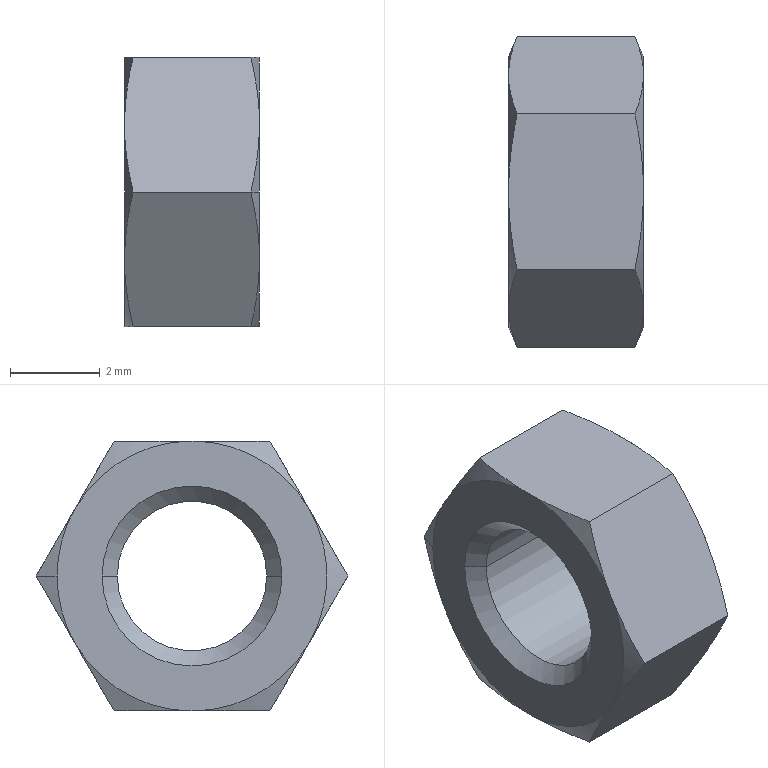Part | SolidWorks | features RefAxis 3, 3DProfileFeature 1, ICE 1, Revolution 1, Scale 1 | 1 solid | 28 faces | box 3 x 6.928 x 6 mm | volume 65.89 mm3 | cone 18 | plane 8 | cylinder 2 | commonest cylinder face diameters 3.324 x2
STEP:
#1=CARTESIAN_POINT('',(1.162,1.662,0.));
#2=VERTEX_POINT('',#1);
#3=CARTESIAN_POINT('',(1.162,-1.662,0.));
#4=VERTEX_POINT('',#3);
#5=CARTESIAN_POINT('',(1.162,0.,0.));
#6=DIRECTION('',(-1.,0.,0.));
#7=DIRECTION('',(0.,-1.,0.));
#8=AXIS2_PLACEMENT_3D('',#5,#6,#7);
#9=CIRCLE('',#8,1.662);
#10=EDGE_CURVE('',#2,#4,#9,.T.);
#11=ORIENTED_EDGE('',*,*,#10,.T.);
#12=CARTESIAN_POINT('',(1.5,-2.,0.));
#13=VERTEX_POINT('',#12);
#14=CARTESIAN_POINT('',(1.162,-1.662,0.));
#15=DIRECTION('',(0.7071,-0.7071,0.));
#16=VECTOR('',#15,1000.);
#17=LINE('',#14,#16);
#18=EDGE_CURVE('',#4,#13,#17,.T.);
#19=ORIENTED_EDGE('',*,*,#18,.T.);
#20=CARTESIAN_POINT('',(1.5,2.,0.));
#21=VERTEX_POINT('',#20);
#22=CARTESIAN_POINT('',(1.5,0.,0.));
#23=DIRECTION('',(-1.,0.,0.));
#24=DIRECTION('',(0.,-1.,0.));
#25=AXIS2_PLACEMENT_3D('',#22,#23,#24);
#26=CIRCLE('',#25,2.);
#27=EDGE_CURVE('',#21,#13,#26,.T.);
#28=ORIENTED_EDGE('',*,*,#27,.F.);
#29=CARTESIAN_POINT('',(1.162,1.662,0.));
#30=DIRECTION('',(0.7071,0.7071,0.));
#31=VECTOR('',#30,1000.);
#32=LINE('',#29,#31);
#33=EDGE_CURVE('',#2,#21,#32,.T.);
#34=ORIENTED_EDGE('',*,*,#33,.F.);
#35=EDGE_LOOP('',(#11,#19,#28,#34));
#36=FACE_OUTER_BOUND('',#35,.T.);
#37=CARTESIAN_POINT('',(1.162,0.,0.));
#38=DIRECTION('',(1.,0.,0.));
#39=DIRECTION('',(0.,1.,0.));
#40=AXIS2_PLACEMENT_3D('',#37,#38,#39);
#41=CONICAL_SURFACE('',#40,1.662,0.7854);
#42=ADVANCED_FACE('',(#36),#41,.F.);
#43=ORIENTED_EDGE('',*,*,#10,.F.);
#44=CARTESIAN_POINT('',(-1.162,1.662,0.));
#45=VERTEX_POINT('',#44);
#46=CARTESIAN_POINT('',(1.5,1.662,0.));
#47=DIRECTION('',(-1.,0.,0.));
#48=VECTOR('',#47,1000.);
#49=LINE('',#46,#48);
#50=EDGE_CURVE('',#2,#45,#49,.T.);
#51=ORIENTED_EDGE('',*,*,#50,.T.);
#52=CARTESIAN_POINT('',(-1.162,-1.662,0.));
#53=VERTEX_POINT('',#52);
#54=CARTESIAN_POINT('',(-1.162,0.,0.));
#55=DIRECTION('',(-1.,0.,0.));
#56=DIRECTION('',(0.,-1.,0.));
#57=AXIS2_PLACEMENT_3D('',#54,#55,#56);
#58=CIRCLE('',#57,1.662);
#59=EDGE_CURVE('',#45,#53,#58,.T.);
#60=ORIENTED_EDGE('',*,*,#59,.T.);
#61=CARTESIAN_POINT('',(1.5,-1.662,0.));
#62=DIRECTION('',(-1.,0.,0.));
#63=VECTOR('',#62,1000.);
#64=LINE('',#61,#63);
#65=EDGE_CURVE('',#4,#53,#64,.T.);
#66=ORIENTED_EDGE('',*,*,#65,.F.);
#67=EDGE_LOOP('',(#43,#51,#60,#66));
#68=FACE_OUTER_BOUND('',#67,.T.);
#69=CARTESIAN_POINT('',(1.5,0.,0.));
#70=DIRECTION('',(-1.,0.,0.));
#71=DIRECTION('',(0.,-1.,0.));
#72=AXIS2_PLACEMENT_3D('',#69,#70,#71);
#73=CYLINDRICAL_SURFACE('',#72,1.662);
#74=ADVANCED_FACE('',(#68),#73,.F.);
#75=ORIENTED_EDGE('',*,*,#59,.F.);
#76=CARTESIAN_POINT('',(-1.5,2.,0.));
#77=VERTEX_POINT('',#76);
#78=CARTESIAN_POINT('',(-1.5,2.,0.));
#79=DIRECTION('',(-0.7071,0.7071,0.));
#80=VECTOR('',#79,1000.);
#81=LINE('',#78,#80);
#82=EDGE_CURVE('',#45,#77,#81,.T.);
#83=ORIENTED_EDGE('',*,*,#82,.T.);
#84=CARTESIAN_POINT('',(-1.5,-2.,0.));
#85=VERTEX_POINT('',#84);
#86=CARTESIAN_POINT('',(-1.5,0.,0.));
#87=DIRECTION('',(-1.,0.,0.));
#88=DIRECTION('',(0.,-1.,0.));
#89=AXIS2_PLACEMENT_3D('',#86,#87,#88);
#90=CIRCLE('',#89,2.);
#91=EDGE_CURVE('',#77,#85,#90,.T.);
#92=ORIENTED_EDGE('',*,*,#91,.T.);
#93=CARTESIAN_POINT('',(-1.5,-2.,0.));
#94=DIRECTION('',(-0.7071,-0.7071,0.));
#95=VECTOR('',#94,1000.);
#96=LINE('',#93,#95);
#97=EDGE_CURVE('',#53,#85,#96,.T.);
#98=ORIENTED_EDGE('',*,*,#97,.F.);
#99=EDGE_LOOP('',(#75,#83,#92,#98));
#100=FACE_OUTER_BOUND('',#99,.T.);
#101=CARTESIAN_POINT('',(-1.5,0.,0.));
#102=DIRECTION('',(-1.,0.,0.));
#103=DIRECTION('',(0.,-1.,0.));
#104=AXIS2_PLACEMENT_3D('',#101,#102,#103);
#105=CONICAL_SURFACE('',#104,2.,0.7854);
#106=ADVANCED_FACE('',(#100),#105,.F.);
#107=CARTESIAN_POINT('',(1.5,-2.598,-1.5));
#108=VERTEX_POINT('',#107);
#109=CARTESIAN_POINT('',(1.5,-3.,0.));
#110=VERTEX_POINT('',#109);
#111=CARTESIAN_POINT('',(1.5,0.,0.));
#112=DIRECTION('',(-1.,0.,0.));
#113=DIRECTION('',(0.,-1.,0.));
#114=AXIS2_PLACEMENT_3D('',#111,#112,#113);
#115=CIRCLE('',#114,3.);
#116=EDGE_CURVE('',#108,#110,#115,.T.);
#117=ORIENTED_EDGE('',*,*,#116,.T.);
#118=CARTESIAN_POINT('',(1.308,-3.464,0.));
#119=VERTEX_POINT('',#118);
#120=CARTESIAN_POINT('',(1.5,-3.,0.));
#121=DIRECTION('',(-0.3827,-0.9239,0.));
#122=VECTOR('',#121,1000.);
#123=LINE('',#120,#122);
#124=EDGE_CURVE('',#110,#119,#123,.T.);
#125=ORIENTED_EDGE('',*,*,#124,.T.);
#126=CARTESIAN_POINT('',(1.5,-2.598,-1.5));
#127=CARTESIAN_POINT('',(1.5,-2.742,-1.25));
#128=CARTESIAN_POINT('',(1.482,-2.887,-1.));
#129=CARTESIAN_POINT('',(1.416,-3.176,-0.499));
#130=CARTESIAN_POINT('',(1.367,-3.321,-0.2483));
#131=CARTESIAN_POINT('',(1.308,-3.464,0.));
#132=B_SPLINE_CURVE_WITH_KNOTS('',3,(#126,#127,#128,#129,#130,#131),.UNSPECIFIED.,.F.,.F.,(4,2,4),(0.001738,0.002602,0.003466),.UNSPECIFIED.);
#133=EDGE_CURVE('',#108,#119,#132,.T.);
#134=ORIENTED_EDGE('',*,*,#133,.F.);
#135=EDGE_LOOP('',(#117,#125,#134));
#136=FACE_OUTER_BOUND('',#135,.T.);
#137=CARTESIAN_POINT('',(1.5,0.,0.));
#138=DIRECTION('',(-1.,0.,0.));
#139=DIRECTION('',(0.,-1.,0.));
#140=AXIS2_PLACEMENT_3D('',#137,#138,#139);
#141=CONICAL_SURFACE('',#140,3.,1.178);
#142=ADVANCED_FACE('',(#136),#141,.T.);
#143=CARTESIAN_POINT('',(-1.5,3.,0.));
#144=VERTEX_POINT('',#143);
#145=CARTESIAN_POINT('',(-1.5,2.598,-1.5));
#146=VERTEX_POINT('',#145);
#147=CARTESIAN_POINT('',(-1.5,0.,0.));
#148=DIRECTION('',(-1.,0.,0.));
#149=DIRECTION('',(0.,-1.,0.));
#150=AXIS2_PLACEMENT_3D('',#147,#148,#149);
#151=CIRCLE('',#150,3.);
#152=EDGE_CURVE('',#144,#146,#151,.T.);
#153=ORIENTED_EDGE('',*,*,#152,.F.);
#154=CARTESIAN_POINT('',(-1.308,3.464,0.));
#155=VERTEX_POINT('',#154);
#156=CARTESIAN_POINT('',(0.,6.621,0.));
#157=DIRECTION('',(0.3827,0.9239,0.));
#158=VECTOR('',#157,1000.);
#159=LINE('',#156,#158);
#160=EDGE_CURVE('',#144,#155,#159,.T.);
#161=ORIENTED_EDGE('',*,*,#160,.T.);
#162=CARTESIAN_POINT('',(-1.5,2.598,-1.5));
#163=CARTESIAN_POINT('',(-1.5,2.742,-1.25));
#164=CARTESIAN_POINT('',(-1.482,2.887,-1.));
#165=CARTESIAN_POINT('',(-1.416,3.176,-0.499));
#166=CARTESIAN_POINT('',(-1.367,3.321,-0.2483));
#167=CARTESIAN_POINT('',(-1.308,3.464,0.));
#168=B_SPLINE_CURVE_WITH_KNOTS('',3,(#162,#163,#164,#165,#166,#167),.UNSPECIFIED.,.F.,.F.,(4,2,4),(0.001738,0.002602,0.003466),.UNSPECIFIED.);
#169=EDGE_CURVE('',#146,#155,#168,.T.);
#170=ORIENTED_EDGE('',*,*,#169,.F.);
#171=EDGE_LOOP('',(#153,#161,#170));
#172=FACE_OUTER_BOUND('',#171,.T.);
#173=CARTESIAN_POINT('',(0.,0.,0.));
#174=DIRECTION('',(1.,0.,0.));
#175=DIRECTION('',(0.,1.,0.));
#176=AXIS2_PLACEMENT_3D('',#173,#174,#175);
#177=CONICAL_SURFACE('',#176,6.621,1.178);
#178=ADVANCED_FACE('',(#172),#177,.T.);
#179=CARTESIAN_POINT('',(-1.308,1.732,-3.));
#180=VERTEX_POINT('',#179);
#181=CARTESIAN_POINT('',(-1.308,1.732,-3.));
#182=CARTESIAN_POINT('',(-1.427,2.02,-2.502));
#183=CARTESIAN_POINT('',(-1.5,2.308,-2.002));
#184=CARTESIAN_POINT('',(-1.5,2.598,-1.5));
#185=B_SPLINE_CURVE_WITH_KNOTS('',3,(#181,#182,#183,#184),.UNSPECIFIED.,.F.,.F.,(4,4),(0.000000116,0.001738),.UNSPECIFIED.);
#186=EDGE_CURVE('',#180,#146,#185,.T.);
#187=ORIENTED_EDGE('',*,*,#186,.F.);
#188=CARTESIAN_POINT('',(-1.5,0.,-3.));
#189=VERTEX_POINT('',#188);
#190=CARTESIAN_POINT('',(-1.5,0.,-3.));
#191=CARTESIAN_POINT('',(-1.5,0.2891,-3.));
#192=CARTESIAN_POINT('',(-1.482,0.5782,-3.));
#193=CARTESIAN_POINT('',(-1.416,1.157,-3.));
#194=CARTESIAN_POINT('',(-1.367,1.447,-3.));
#195=CARTESIAN_POINT('',(-1.308,1.732,-3.));
#196=B_SPLINE_CURVE_WITH_KNOTS('',3,(#190,#191,#192,#193,#194,#195),.UNSPECIFIED.,.F.,.F.,(4,2,4),(0.004788,0.005662,0.006536),.UNSPECIFIED.);
#197=EDGE_CURVE('',#189,#180,#196,.T.);
#198=ORIENTED_EDGE('',*,*,#197,.F.);
#199=CARTESIAN_POINT('',(-1.5,0.,0.));
#200=DIRECTION('',(-1.,0.,0.));
#201=DIRECTION('',(0.,-1.,0.));
#202=AXIS2_PLACEMENT_3D('',#199,#200,#201);
#203=CIRCLE('',#202,3.);
#204=EDGE_CURVE('',#146,#189,#203,.T.);
#205=ORIENTED_EDGE('',*,*,#204,.F.);
#206=EDGE_LOOP('',(#187,#198,#205));
#207=FACE_OUTER_BOUND('',#206,.T.);
#208=CARTESIAN_POINT('',(0.,0.,0.));
#209=DIRECTION('',(1.,0.,0.));
#210=DIRECTION('',(0.,1.,0.));
#211=AXIS2_PLACEMENT_3D('',#208,#209,#210);
#212=CONICAL_SURFACE('',#211,6.621,1.178);
#213=ADVANCED_FACE('',(#207),#212,.T.);
#214=ORIENTED_EDGE('',*,*,#160,.F.);
#215=CARTESIAN_POINT('',(-1.5,2.598,1.5));
#216=VERTEX_POINT('',#215);
#217=CARTESIAN_POINT('',(-1.5,0.,0.));
#218=DIRECTION('',(-1.,0.,0.));
#219=DIRECTION('',(0.,-1.,0.));
#220=AXIS2_PLACEMENT_3D('',#217,#218,#219);
#221=CIRCLE('',#220,3.);
#222=EDGE_CURVE('',#216,#144,#221,.T.);
#223=ORIENTED_EDGE('',*,*,#222,.F.);
#224=CARTESIAN_POINT('',(-1.308,3.464,0.));
#225=CARTESIAN_POINT('',(-1.427,3.176,0.4982));
#226=CARTESIAN_POINT('',(-1.5,2.888,0.9979));
#227=CARTESIAN_POINT('',(-1.5,2.598,1.5));
#228=B_SPLINE_CURVE_WITH_KNOTS('',3,(#224,#225,#226,#227),.UNSPECIFIED.,.F.,.F.,(4,4),(0.000000116,0.001738),.UNSPECIFIED.);
#229=EDGE_CURVE('',#155,#216,#228,.T.);
#230=ORIENTED_EDGE('',*,*,#229,.F.);
#231=EDGE_LOOP('',(#214,#223,#230));
#232=FACE_OUTER_BOUND('',#231,.T.);
#233=CARTESIAN_POINT('',(0.,0.,0.));
#234=DIRECTION('',(1.,0.,0.));
#235=DIRECTION('',(0.,1.,0.));
#236=AXIS2_PLACEMENT_3D('',#233,#234,#235);
#237=CONICAL_SURFACE('',#236,6.621,1.178);
#238=ADVANCED_FACE('',(#232),#237,.T.);
#239=CARTESIAN_POINT('',(-1.308,1.732,3.));
#240=VERTEX_POINT('',#239);
#241=CARTESIAN_POINT('',(-1.5,2.598,1.5));
#242=CARTESIAN_POINT('',(-1.5,2.454,1.75));
#243=CARTESIAN_POINT('',(-1.482,2.31,2.));
#244=CARTESIAN_POINT('',(-1.416,2.02,2.501));
#245=CARTESIAN_POINT('',(-1.367,1.875,2.752));
#246=CARTESIAN_POINT('',(-1.308,1.732,3.));
#247=B_SPLINE_CURVE_WITH_KNOTS('',3,(#241,#242,#243,#244,#245,#246),.UNSPECIFIED.,.F.,.F.,(4,2,4),(0.001738,0.002602,0.003466),.UNSPECIFIED.);
#248=EDGE_CURVE('',#216,#240,#247,.T.);
#249=ORIENTED_EDGE('',*,*,#248,.F.);
#250=CARTESIAN_POINT('',(-1.5,0.,3.));
#251=VERTEX_POINT('',#250);
#252=CARTESIAN_POINT('',(-1.5,0.,0.));
#253=DIRECTION('',(-1.,0.,0.));
#254=DIRECTION('',(0.,-1.,0.));
#255=AXIS2_PLACEMENT_3D('',#252,#253,#254);
#256=CIRCLE('',#255,3.);
#257=EDGE_CURVE('',#251,#216,#256,.T.);
#258=ORIENTED_EDGE('',*,*,#257,.F.);
#259=CARTESIAN_POINT('',(-1.308,1.732,3.));
#260=CARTESIAN_POINT('',(-1.367,1.447,3.));
#261=CARTESIAN_POINT('',(-1.416,1.157,3.));
#262=CARTESIAN_POINT('',(-1.482,0.5782,3.));
#263=CARTESIAN_POINT('',(-1.5,0.2891,3.));
#264=CARTESIAN_POINT('',(-1.5,0.,3.));
#265=B_SPLINE_CURVE_WITH_KNOTS('',3,(#259,#260,#261,#262,#263,#264),.UNSPECIFIED.,.F.,.F.,(4,2,4),(0.007219,0.008087,0.008956),.UNSPECIFIED.);
#266=EDGE_CURVE('',#240,#251,#265,.T.);
#267=ORIENTED_EDGE('',*,*,#266,.F.);
#268=EDGE_LOOP('',(#249,#258,#267));
#269=FACE_OUTER_BOUND('',#268,.T.);
#270=CARTESIAN_POINT('',(0.,0.,0.));
#271=DIRECTION('',(1.,0.,0.));
#272=DIRECTION('',(0.,1.,0.));
#273=AXIS2_PLACEMENT_3D('',#270,#271,#272);
#274=CONICAL_SURFACE('',#273,6.621,1.178);
#275=ADVANCED_FACE('',(#269),#274,.T.);
#276=CARTESIAN_POINT('',(-1.308,-1.732,-3.));
#277=VERTEX_POINT('',#276);
#278=CARTESIAN_POINT('',(-1.308,-1.732,-3.));
#279=CARTESIAN_POINT('',(-1.367,-1.446,-3.));
#280=CARTESIAN_POINT('',(-1.416,-1.156,-3.));
#281=CARTESIAN_POINT('',(-1.482,-0.5781,-3.));
#282=CARTESIAN_POINT('',(-1.5,-0.2891,-3.));
#283=CARTESIAN_POINT('',(-1.5,0.,-3.));
#284=B_SPLINE_CURVE_WITH_KNOTS('',3,(#278,#279,#280,#281,#282,#283),.UNSPECIFIED.,.F.,.F.,(4,2,4),(0.00304,0.003914,0.004788),.UNSPECIFIED.);
#285=EDGE_CURVE('',#277,#189,#284,.T.);
#286=ORIENTED_EDGE('',*,*,#285,.F.);
#287=CARTESIAN_POINT('',(-1.5,-2.598,-1.5));
#288=VERTEX_POINT('',#287);
#289=CARTESIAN_POINT('',(-1.5,-2.598,-1.5));
#290=CARTESIAN_POINT('',(-1.5,-2.454,-1.75));
#291=CARTESIAN_POINT('',(-1.482,-2.31,-2.));
#292=CARTESIAN_POINT('',(-1.416,-2.02,-2.501));
#293=CARTESIAN_POINT('',(-1.367,-1.875,-2.752));
#294=CARTESIAN_POINT('',(-1.308,-1.732,-3.));
#295=B_SPLINE_CURVE_WITH_KNOTS('',3,(#289,#290,#291,#292,#293,#294),.UNSPECIFIED.,.F.,.F.,(4,2,4),(0.001738,0.002602,0.003466),.UNSPECIFIED.);
#296=EDGE_CURVE('',#288,#277,#295,.T.);
#297=ORIENTED_EDGE('',*,*,#296,.F.);
#298=CARTESIAN_POINT('',(-1.5,0.,0.));
#299=DIRECTION('',(-1.,0.,0.));
#300=DIRECTION('',(0.,-1.,0.));
#301=AXIS2_PLACEMENT_3D('',#298,#299,#300);
#302=CIRCLE('',#301,3.);
#303=EDGE_CURVE('',#189,#288,#302,.T.);
#304=ORIENTED_EDGE('',*,*,#303,.F.);
#305=EDGE_LOOP('',(#286,#297,#304));
#306=FACE_OUTER_BOUND('',#305,.T.);
#307=CARTESIAN_POINT('',(0.,0.,0.));
#308=DIRECTION('',(1.,0.,0.));
#309=DIRECTION('',(0.,1.,0.));
#310=AXIS2_PLACEMENT_3D('',#307,#308,#309);
#311=CONICAL_SURFACE('',#310,6.621,1.178);
#312=ADVANCED_FACE('',(#306),#311,.T.);
#313=CARTESIAN_POINT('',(-1.308,-1.732,3.));
#314=VERTEX_POINT('',#313);
#315=CARTESIAN_POINT('',(-1.5,0.,3.));
#316=CARTESIAN_POINT('',(-1.5,-0.2891,3.));
#317=CARTESIAN_POINT('',(-1.482,-0.5781,3.));
#318=CARTESIAN_POINT('',(-1.416,-1.156,3.));
#319=CARTESIAN_POINT('',(-1.367,-1.446,3.));
#320=CARTESIAN_POINT('',(-1.308,-1.732,3.));
#321=B_SPLINE_CURVE_WITH_KNOTS('',3,(#315,#316,#317,#318,#319,#320),.UNSPECIFIED.,.F.,.F.,(4,2,4),(0.008956,0.009825,0.01069),.UNSPECIFIED.);
#322=EDGE_CURVE('',#251,#314,#321,.T.);
#323=ORIENTED_EDGE('',*,*,#322,.F.);
#324=CARTESIAN_POINT('',(-1.5,-2.598,1.5));
#325=VERTEX_POINT('',#324);
#326=CARTESIAN_POINT('',(-1.5,0.,0.));
#327=DIRECTION('',(-1.,0.,0.));
#328=DIRECTION('',(0.,-1.,0.));
#329=AXIS2_PLACEMENT_3D('',#326,#327,#328);
#330=CIRCLE('',#329,3.);
#331=EDGE_CURVE('',#325,#251,#330,.T.);
#332=ORIENTED_EDGE('',*,*,#331,.F.);
#333=CARTESIAN_POINT('',(-1.308,-1.732,3.));
#334=CARTESIAN_POINT('',(-1.427,-2.02,2.502));
#335=CARTESIAN_POINT('',(-1.5,-2.308,2.002));
#336=CARTESIAN_POINT('',(-1.5,-2.598,1.5));
#337=B_SPLINE_CURVE_WITH_KNOTS('',3,(#333,#334,#335,#336),.UNSPECIFIED.,.F.,.F.,(4,4),(0.000000116,0.001738),.UNSPECIFIED.);
#338=EDGE_CURVE('',#314,#325,#337,.T.);
#339=ORIENTED_EDGE('',*,*,#338,.F.);
#340=EDGE_LOOP('',(#323,#332,#339));
#341=FACE_OUTER_BOUND('',#340,.T.);
#342=CARTESIAN_POINT('',(0.,0.,0.));
#343=DIRECTION('',(1.,0.,0.));
#344=DIRECTION('',(0.,1.,0.));
#345=AXIS2_PLACEMENT_3D('',#342,#343,#344);
#346=CONICAL_SURFACE('',#345,6.621,1.178);
#347=ADVANCED_FACE('',(#341),#346,.T.);
#348=CARTESIAN_POINT('',(-1.308,-3.464,0.));
#349=VERTEX_POINT('',#348);
#350=CARTESIAN_POINT('',(-1.308,-3.464,0.));
#351=CARTESIAN_POINT('',(-1.427,-3.176,-0.4982));
#352=CARTESIAN_POINT('',(-1.5,-2.888,-0.9979));
#353=CARTESIAN_POINT('',(-1.5,-2.598,-1.5));
#354=B_SPLINE_CURVE_WITH_KNOTS('',3,(#350,#351,#352,#353),.UNSPECIFIED.,.F.,.F.,(4,4),(0.000000116,0.001738),.UNSPECIFIED.);
#355=EDGE_CURVE('',#349,#288,#354,.T.);
#356=ORIENTED_EDGE('',*,*,#355,.F.);
#357=CARTESIAN_POINT('',(-1.5,-2.598,1.5));
#358=CARTESIAN_POINT('',(-1.5,-2.742,1.25));
#359=CARTESIAN_POINT('',(-1.482,-2.887,1.));
#360=CARTESIAN_POINT('',(-1.416,-3.176,0.499));
#361=CARTESIAN_POINT('',(-1.367,-3.321,0.2483));
#362=CARTESIAN_POINT('',(-1.308,-3.464,0.));
#363=B_SPLINE_CURVE_WITH_KNOTS('',3,(#357,#358,#359,#360,#361,#362),.UNSPECIFIED.,.F.,.F.,(4,2,4),(0.001738,0.002602,0.003466),.UNSPECIFIED.);
#364=EDGE_CURVE('',#325,#349,#363,.T.);
#365=ORIENTED_EDGE('',*,*,#364,.F.);
#366=CARTESIAN_POINT('',(-1.5,0.,0.));
#367=DIRECTION('',(-1.,0.,0.));
#368=DIRECTION('',(0.,-1.,0.));
#369=AXIS2_PLACEMENT_3D('',#366,#367,#368);
#370=CIRCLE('',#369,3.);
#371=EDGE_CURVE('',#288,#325,#370,.T.);
#372=ORIENTED_EDGE('',*,*,#371,.F.);
#373=EDGE_LOOP('',(#356,#365,#372));
#374=FACE_OUTER_BOUND('',#373,.T.);
#375=CARTESIAN_POINT('',(0.,0.,0.));
#376=DIRECTION('',(1.,0.,0.));
#377=DIRECTION('',(0.,1.,0.));
#378=AXIS2_PLACEMENT_3D('',#375,#376,#377);
#379=CONICAL_SURFACE('',#378,6.621,1.178);
#380=ADVANCED_FACE('',(#374),#379,.T.);
#381=CARTESIAN_POINT('',(1.308,-1.732,3.));
#382=VERTEX_POINT('',#381);
#383=CARTESIAN_POINT('',(1.5,0.,3.));
#384=VERTEX_POINT('',#383);
#385=CARTESIAN_POINT('',(1.308,-1.732,3.));
#386=CARTESIAN_POINT('',(1.367,-1.446,3.));
#387=CARTESIAN_POINT('',(1.416,-1.156,3.));
#388=CARTESIAN_POINT('',(1.482,-0.5781,3.));
#389=CARTESIAN_POINT('',(1.5,-0.2891,3.));
#390=CARTESIAN_POINT('',(1.5,0.,3.));
#391=B_SPLINE_CURVE_WITH_KNOTS('',3,(#385,#386,#387,#388,#389,#390),.UNSPECIFIED.,.F.,.F.,(4,2,4),(0.00304,0.003914,0.004788),.UNSPECIFIED.);
#392=EDGE_CURVE('',#382,#384,#391,.T.);
#393=ORIENTED_EDGE('',*,*,#392,.F.);
#394=CARTESIAN_POINT('',(1.5,-2.598,1.5));
#395=VERTEX_POINT('',#394);
#396=CARTESIAN_POINT('',(1.5,-2.598,1.5));
#397=CARTESIAN_POINT('',(1.5,-2.454,1.75));
#398=CARTESIAN_POINT('',(1.482,-2.31,2.));
#399=CARTESIAN_POINT('',(1.416,-2.02,2.501));
#400=CARTESIAN_POINT('',(1.367,-1.875,2.752));
#401=CARTESIAN_POINT('',(1.308,-1.732,3.));
#402=B_SPLINE_CURVE_WITH_KNOTS('',3,(#396,#397,#398,#399,#400,#401),.UNSPECIFIED.,.F.,.F.,(4,2,4),(0.001738,0.002602,0.003466),.UNSPECIFIED.);
#403=EDGE_CURVE('',#395,#382,#402,.T.);
#404=ORIENTED_EDGE('',*,*,#403,.F.);
#405=CARTESIAN_POINT('',(1.5,0.,0.));
#406=DIRECTION('',(-1.,0.,0.));
#407=DIRECTION('',(0.,-1.,0.));
#408=AXIS2_PLACEMENT_3D('',#405,#406,#407);
#409=CIRCLE('',#408,3.);
#410=EDGE_CURVE('',#395,#384,#409,.T.);
#411=ORIENTED_EDGE('',*,*,#410,.T.);
#412=EDGE_LOOP('',(#393,#404,#411));
#413=FACE_OUTER_BOUND('',#412,.T.);
#414=CARTESIAN_POINT('',(1.5,0.,0.));
#415=DIRECTION('',(-1.,0.,0.));
#416=DIRECTION('',(0.,-1.,0.));
#417=AXIS2_PLACEMENT_3D('',#414,#415,#416);
#418=CONICAL_SURFACE('',#417,3.,1.178);
#419=ADVANCED_FACE('',(#413),#418,.T.);
#420=CARTESIAN_POINT('',(1.308,1.732,3.));
#421=VERTEX_POINT('',#420);
#422=CARTESIAN_POINT('',(1.5,0.,3.));
#423=CARTESIAN_POINT('',(1.5,0.2891,3.));
#424=CARTESIAN_POINT('',(1.482,0.5782,3.));
#425=CARTESIAN_POINT('',(1.416,1.157,3.));
#426=CARTESIAN_POINT('',(1.367,1.447,3.));
#427=CARTESIAN_POINT('',(1.308,1.732,3.));
#428=B_SPLINE_CURVE_WITH_KNOTS('',3,(#422,#423,#424,#425,#426,#427),.UNSPECIFIED.,.F.,.F.,(4,2,4),(0.004788,0.005662,0.006536),.UNSPECIFIED.);
#429=EDGE_CURVE('',#384,#421,#428,.T.);
#430=ORIENTED_EDGE('',*,*,#429,.F.);
#431=CARTESIAN_POINT('',(1.5,2.598,1.5));
#432=VERTEX_POINT('',#431);
#433=CARTESIAN_POINT('',(1.5,0.,0.));
#434=DIRECTION('',(-1.,0.,0.));
#435=DIRECTION('',(0.,-1.,0.));
#436=AXIS2_PLACEMENT_3D('',#433,#434,#435);
#437=CIRCLE('',#436,3.);
#438=EDGE_CURVE('',#384,#432,#437,.T.);
#439=ORIENTED_EDGE('',*,*,#438,.T.);
#440=CARTESIAN_POINT('',(1.308,1.732,3.));
#441=CARTESIAN_POINT('',(1.427,2.02,2.502));
#442=CARTESIAN_POINT('',(1.5,2.308,2.002));
#443=CARTESIAN_POINT('',(1.5,2.598,1.5));
#444=B_SPLINE_CURVE_WITH_KNOTS('',3,(#440,#441,#442,#443),.UNSPECIFIED.,.F.,.F.,(4,4),(0.000000116,0.001738),.UNSPECIFIED.);
#445=EDGE_CURVE('',#421,#432,#444,.T.);
#446=ORIENTED_EDGE('',*,*,#445,.F.);
#447=EDGE_LOOP('',(#430,#439,#446));
#448=FACE_OUTER_BOUND('',#447,.T.);
#449=CARTESIAN_POINT('',(1.5,0.,0.));
#450=DIRECTION('',(-1.,0.,0.));
#451=DIRECTION('',(0.,-1.,0.));
#452=AXIS2_PLACEMENT_3D('',#449,#450,#451);
#453=CONICAL_SURFACE('',#452,3.,1.178);
#454=ADVANCED_FACE('',(#448),#453,.T.);
#455=CARTESIAN_POINT('',(1.308,3.464,0.));
#456=VERTEX_POINT('',#455);
#457=CARTESIAN_POINT('',(1.5,2.598,1.5));
#458=CARTESIAN_POINT('',(1.5,2.742,1.25));
#459=CARTESIAN_POINT('',(1.482,2.887,1.));
#460=CARTESIAN_POINT('',(1.416,3.176,0.499));
#461=CARTESIAN_POINT('',(1.367,3.321,0.2483));
#462=CARTESIAN_POINT('',(1.308,3.464,0.));
#463=B_SPLINE_CURVE_WITH_KNOTS('',3,(#457,#458,#459,#460,#461,#462),.UNSPECIFIED.,.F.,.F.,(4,2,4),(0.001738,0.002602,0.003466),.UNSPECIFIED.);
#464=EDGE_CURVE('',#432,#456,#463,.T.);
#465=ORIENTED_EDGE('',*,*,#464,.F.);
#466=CARTESIAN_POINT('',(1.5,2.598,-1.5));
#467=VERTEX_POINT('',#466);
#468=CARTESIAN_POINT('',(1.5,0.,0.));
#469=DIRECTION('',(-1.,0.,0.));
#470=DIRECTION('',(0.,-1.,0.));
#471=AXIS2_PLACEMENT_3D('',#468,#469,#470);
#472=CIRCLE('',#471,3.);
#473=EDGE_CURVE('',#432,#467,#472,.T.);
#474=ORIENTED_EDGE('',*,*,#473,.T.);
#475=CARTESIAN_POINT('',(1.308,3.464,0.));
#476=CARTESIAN_POINT('',(1.427,3.176,-0.4982));
#477=CARTESIAN_POINT('',(1.5,2.888,-0.9979));
#478=CARTESIAN_POINT('',(1.5,2.598,-1.5));
#479=B_SPLINE_CURVE_WITH_KNOTS('',3,(#475,#476,#477,#478),.UNSPECIFIED.,.F.,.F.,(4,4),(0.000000116,0.001738),.UNSPECIFIED.);
#480=EDGE_CURVE('',#456,#467,#479,.T.);
#481=ORIENTED_EDGE('',*,*,#480,.F.);
#482=EDGE_LOOP('',(#465,#474,#481));
#483=FACE_OUTER_BOUND('',#482,.T.);
#484=CARTESIAN_POINT('',(1.5,0.,0.));
#485=DIRECTION('',(-1.,0.,0.));
#486=DIRECTION('',(0.,-1.,0.));
#487=AXIS2_PLACEMENT_3D('',#484,#485,#486);
#488=CONICAL_SURFACE('',#487,3.,1.178);
#489=ADVANCED_FACE('',(#483),#488,.T.);
#490=CARTESIAN_POINT('',(1.308,1.732,-3.));
#491=VERTEX_POINT('',#490);
#492=CARTESIAN_POINT('',(1.5,2.598,-1.5));
#493=CARTESIAN_POINT('',(1.5,2.454,-1.75));
#494=CARTESIAN_POINT('',(1.482,2.31,-2.));
#495=CARTESIAN_POINT('',(1.416,2.02,-2.501));
#496=CARTESIAN_POINT('',(1.367,1.875,-2.752));
#497=CARTESIAN_POINT('',(1.308,1.732,-3.));
#498=B_SPLINE_CURVE_WITH_KNOTS('',3,(#492,#493,#494,#495,#496,#497),.UNSPECIFIED.,.F.,.F.,(4,2,4),(0.001738,0.002602,0.003466),.UNSPECIFIED.);
#499=EDGE_CURVE('',#467,#491,#498,.T.);
#500=ORIENTED_EDGE('',*,*,#499,.F.);
#501=CARTESIAN_POINT('',(1.5,0.,-3.));
#502=VERTEX_POINT('',#501);
#503=CARTESIAN_POINT('',(1.5,0.,0.));
#504=DIRECTION('',(-1.,0.,0.));
#505=DIRECTION('',(0.,-1.,0.));
#506=AXIS2_PLACEMENT_3D('',#503,#504,#505);
#507=CIRCLE('',#506,3.);
#508=EDGE_CURVE('',#467,#502,#507,.T.);
#509=ORIENTED_EDGE('',*,*,#508,.T.);
#510=CARTESIAN_POINT('',(1.308,1.732,-3.));
#511=CARTESIAN_POINT('',(1.367,1.447,-3.));
#512=CARTESIAN_POINT('',(1.416,1.157,-3.));
#513=CARTESIAN_POINT('',(1.482,0.5782,-3.));
#514=CARTESIAN_POINT('',(1.5,0.2891,-3.));
#515=CARTESIAN_POINT('',(1.5,0.,-3.));
#516=B_SPLINE_CURVE_WITH_KNOTS('',3,(#510,#511,#512,#513,#514,#515),.UNSPECIFIED.,.F.,.F.,(4,2,4),(0.007219,0.008087,0.008956),.UNSPECIFIED.);
#517=EDGE_CURVE('',#491,#502,#516,.T.);
#518=ORIENTED_EDGE('',*,*,#517,.F.);
#519=EDGE_LOOP('',(#500,#509,#518));
#520=FACE_OUTER_BOUND('',#519,.T.);
#521=CARTESIAN_POINT('',(1.5,0.,0.));
#522=DIRECTION('',(-1.,0.,0.));
#523=DIRECTION('',(0.,-1.,0.));
#524=AXIS2_PLACEMENT_3D('',#521,#522,#523);
#525=CONICAL_SURFACE('',#524,3.,1.178);
#526=ADVANCED_FACE('',(#520),#525,.T.);
#527=CARTESIAN_POINT('',(1.308,-1.732,-3.));
#528=VERTEX_POINT('',#527);
#529=CARTESIAN_POINT('',(1.5,0.,-3.));
#530=CARTESIAN_POINT('',(1.5,-0.2891,-3.));
#531=CARTESIAN_POINT('',(1.482,-0.5781,-3.));
#532=CARTESIAN_POINT('',(1.416,-1.156,-3.));
#533=CARTESIAN_POINT('',(1.367,-1.446,-3.));
#534=CARTESIAN_POINT('',(1.308,-1.732,-3.));
#535=B_SPLINE_CURVE_WITH_KNOTS('',3,(#529,#530,#531,#532,#533,#534),.UNSPECIFIED.,.F.,.F.,(4,2,4),(0.008956,0.009825,0.01069),.UNSPECIFIED.);
#536=EDGE_CURVE('',#502,#528,#535,.T.);
#537=ORIENTED_EDGE('',*,*,#536,.F.);
#538=CARTESIAN_POINT('',(1.5,0.,0.));
#539=DIRECTION('',(-1.,0.,0.));
#540=DIRECTION('',(0.,-1.,0.));
#541=AXIS2_PLACEMENT_3D('',#538,#539,#540);
#542=CIRCLE('',#541,3.);
#543=EDGE_CURVE('',#502,#108,#542,.T.);
#544=ORIENTED_EDGE('',*,*,#543,.T.);
#545=CARTESIAN_POINT('',(1.308,-1.732,-3.));
#546=CARTESIAN_POINT('',(1.427,-2.02,-2.502));
#547=CARTESIAN_POINT('',(1.5,-2.308,-2.002));
#548=CARTESIAN_POINT('',(1.5,-2.598,-1.5));
#549=B_SPLINE_CURVE_WITH_KNOTS('',3,(#545,#546,#547,#548),.UNSPECIFIED.,.F.,.F.,(4,4),(0.000000116,0.001738),.UNSPECIFIED.);
#550=EDGE_CURVE('',#528,#108,#549,.T.);
#551=ORIENTED_EDGE('',*,*,#550,.F.);
#552=EDGE_LOOP('',(#537,#544,#551));
#553=FACE_OUTER_BOUND('',#552,.T.);
#554=CARTESIAN_POINT('',(1.5,0.,0.));
#555=DIRECTION('',(-1.,0.,0.));
#556=DIRECTION('',(0.,-1.,0.));
#557=AXIS2_PLACEMENT_3D('',#554,#555,#556);
#558=CONICAL_SURFACE('',#557,3.,1.178);
#559=ADVANCED_FACE('',(#553),#558,.T.);
#560=ORIENTED_EDGE('',*,*,#124,.F.);
#561=CARTESIAN_POINT('',(1.5,0.,0.));
#562=DIRECTION('',(-1.,0.,0.));
#563=DIRECTION('',(0.,-1.,0.));
#564=AXIS2_PLACEMENT_3D('',#561,#562,#563);
#565=CIRCLE('',#564,3.);
#566=EDGE_CURVE('',#110,#395,#565,.T.);
#567=ORIENTED_EDGE('',*,*,#566,.T.);
#568=CARTESIAN_POINT('',(1.308,-3.464,0.));
#569=CARTESIAN_POINT('',(1.427,-3.176,0.4982));
#570=CARTESIAN_POINT('',(1.5,-2.888,0.9979));
#571=CARTESIAN_POINT('',(1.5,-2.598,1.5));
#572=B_SPLINE_CURVE_WITH_KNOTS('',3,(#568,#569,#570,#571),.UNSPECIFIED.,.F.,.F.,(4,4),(0.000000116,0.001738),.UNSPECIFIED.);
#573=EDGE_CURVE('',#119,#395,#572,.T.);
#574=ORIENTED_EDGE('',*,*,#573,.F.);
#575=EDGE_LOOP('',(#560,#567,#574));
#576=FACE_OUTER_BOUND('',#575,.T.);
#577=CARTESIAN_POINT('',(1.5,0.,0.));
#578=DIRECTION('',(-1.,0.,0.));
#579=DIRECTION('',(0.,-1.,0.));
#580=AXIS2_PLACEMENT_3D('',#577,#578,#579);
#581=CONICAL_SURFACE('',#580,3.,1.178);
#582=ADVANCED_FACE('',(#576),#581,.T.);
#583=CARTESIAN_POINT('',(-1.5,0.,0.));
#584=DIRECTION('',(-1.,0.,0.));
#585=DIRECTION('',(0.,-1.,0.));
#586=AXIS2_PLACEMENT_3D('',#583,#584,#585);
#587=CIRCLE('',#586,2.);
#588=EDGE_CURVE('',#85,#77,#587,.T.);
#589=ORIENTED_EDGE('',*,*,#588,.F.);
#590=ORIENTED_EDGE('',*,*,#91,.F.);
#591=EDGE_LOOP('',(#589,#590));
#592=FACE_BOUND('',#591,.T.);
#593=ORIENTED_EDGE('',*,*,#331,.T.);
#594=ORIENTED_EDGE('',*,*,#257,.T.);
#595=ORIENTED_EDGE('',*,*,#222,.T.);
#596=ORIENTED_EDGE('',*,*,#152,.T.);
#597=ORIENTED_EDGE('',*,*,#204,.T.);
#598=ORIENTED_EDGE('',*,*,#303,.T.);
#599=ORIENTED_EDGE('',*,*,#371,.T.);
#600=EDGE_LOOP('',(#593,#594,#595,#596,#597,#598,#599));
#601=FACE_OUTER_BOUND('',#600,.T.);
#602=CARTESIAN_POINT('',(-1.5,3.,0.));
#603=DIRECTION('',(1.,0.,0.));
#604=DIRECTION('',(0.,1.,0.));
#605=AXIS2_PLACEMENT_3D('',#602,#603,#604);
#606=PLANE('',#605);
#607=ADVANCED_FACE('',(#592,#601),#606,.F.);
#608=ORIENTED_EDGE('',*,*,#82,.F.);
#609=CARTESIAN_POINT('',(-1.162,0.,0.));
#610=DIRECTION('',(-1.,0.,0.));
#611=DIRECTION('',(0.,-1.,0.));
#612=AXIS2_PLACEMENT_3D('',#609,#610,#611);
#613=CIRCLE('',#612,1.662);
#614=EDGE_CURVE('',#53,#45,#613,.T.);
#615=ORIENTED_EDGE('',*,*,#614,.F.);
#616=ORIENTED_EDGE('',*,*,#97,.T.);
#617=ORIENTED_EDGE('',*,*,#588,.T.);
#618=EDGE_LOOP('',(#608,#615,#616,#617));
#619=FACE_OUTER_BOUND('',#618,.T.);
#620=CARTESIAN_POINT('',(-1.5,0.,0.));
#621=DIRECTION('',(-1.,0.,0.));
#622=DIRECTION('',(0.,-1.,0.));
#623=AXIS2_PLACEMENT_3D('',#620,#621,#622);
#624=CONICAL_SURFACE('',#623,2.,0.7854);
#625=ADVANCED_FACE('',(#619),#624,.F.);
#626=ORIENTED_EDGE('',*,*,#50,.F.);
#627=CARTESIAN_POINT('',(1.162,0.,0.));
#628=DIRECTION('',(-1.,0.,0.));
#629=DIRECTION('',(0.,-1.,0.));
#630=AXIS2_PLACEMENT_3D('',#627,#628,#629);
#631=CIRCLE('',#630,1.662);
#632=EDGE_CURVE('',#4,#2,#631,.T.);
#633=ORIENTED_EDGE('',*,*,#632,.F.);
#634=ORIENTED_EDGE('',*,*,#65,.T.);
#635=ORIENTED_EDGE('',*,*,#614,.T.);
#636=EDGE_LOOP('',(#626,#633,#634,#635));
#637=FACE_OUTER_BOUND('',#636,.T.);
#638=CARTESIAN_POINT('',(1.5,0.,0.));
#639=DIRECTION('',(-1.,0.,0.));
#640=DIRECTION('',(0.,-1.,0.));
#641=AXIS2_PLACEMENT_3D('',#638,#639,#640);
#642=CYLINDRICAL_SURFACE('',#641,1.662);
#643=ADVANCED_FACE('',(#637),#642,.F.);
#644=ORIENTED_EDGE('',*,*,#18,.F.);
#645=ORIENTED_EDGE('',*,*,#632,.T.);
#646=ORIENTED_EDGE('',*,*,#33,.T.);
#647=CARTESIAN_POINT('',(1.5,0.,0.));
#648=DIRECTION('',(-1.,0.,0.));
#649=DIRECTION('',(0.,-1.,0.));
#650=AXIS2_PLACEMENT_3D('',#647,#648,#649);
#651=CIRCLE('',#650,2.);
#652=EDGE_CURVE('',#13,#21,#651,.T.);
#653=ORIENTED_EDGE('',*,*,#652,.F.);
#654=EDGE_LOOP('',(#644,#645,#646,#653));
#655=FACE_OUTER_BOUND('',#654,.T.);
#656=CARTESIAN_POINT('',(1.162,0.,0.));
#657=DIRECTION('',(1.,0.,0.));
#658=DIRECTION('',(0.,1.,0.));
#659=AXIS2_PLACEMENT_3D('',#656,#657,#658);
#660=CONICAL_SURFACE('',#659,1.662,0.7854);
#661=ADVANCED_FACE('',(#655),#660,.F.);
#662=ORIENTED_EDGE('',*,*,#410,.F.);
#663=ORIENTED_EDGE('',*,*,#566,.F.);
#664=ORIENTED_EDGE('',*,*,#116,.F.);
#665=ORIENTED_EDGE('',*,*,#543,.F.);
#666=ORIENTED_EDGE('',*,*,#508,.F.);
#667=ORIENTED_EDGE('',*,*,#473,.F.);
#668=ORIENTED_EDGE('',*,*,#438,.F.);
#669=EDGE_LOOP('',(#662,#663,#664,#665,#666,#667,#668));
#670=FACE_OUTER_BOUND('',#669,.T.);
#671=ORIENTED_EDGE('',*,*,#27,.T.);
#672=ORIENTED_EDGE('',*,*,#652,.T.);
#673=EDGE_LOOP('',(#671,#672));
#674=FACE_BOUND('',#673,.T.);
#675=CARTESIAN_POINT('',(1.5,2.,0.));
#676=DIRECTION('',(-1.,0.,0.));
#677=DIRECTION('',(0.,-1.,0.));
#678=AXIS2_PLACEMENT_3D('',#675,#676,#677);
#679=PLANE('',#678);
#680=ADVANCED_FACE('',(#670,#674),#679,.F.);
#681=ORIENTED_EDGE('',*,*,#266,.T.);
#682=ORIENTED_EDGE('',*,*,#322,.T.);
#683=CARTESIAN_POINT('',(-1.5,-1.732,3.));
#684=DIRECTION('',(1.,0.,0.));
#685=VECTOR('',#684,1000.);
#686=LINE('',#683,#685);
#687=EDGE_CURVE('',#314,#382,#686,.T.);
#688=ORIENTED_EDGE('',*,*,#687,.T.);
#689=ORIENTED_EDGE('',*,*,#392,.T.);
#690=ORIENTED_EDGE('',*,*,#429,.T.);
#691=CARTESIAN_POINT('',(-1.5,1.732,3.));
#692=DIRECTION('',(1.,0.,0.));
#693=VECTOR('',#692,1000.);
#694=LINE('',#691,#693);
#695=EDGE_CURVE('',#240,#421,#694,.T.);
#696=ORIENTED_EDGE('',*,*,#695,.F.);
#697=EDGE_LOOP('',(#681,#682,#688,#689,#690,#696));
#698=FACE_OUTER_BOUND('',#697,.T.);
#699=CARTESIAN_POINT('',(-1.5,1.732,3.));
#700=DIRECTION('',(0.,0.,1.));
#701=DIRECTION('',(0.,-1.,0.));
#702=AXIS2_PLACEMENT_3D('',#699,#700,#701);
#703=PLANE('',#702);
#704=ADVANCED_FACE('',(#698),#703,.T.);
#705=ORIENTED_EDGE('',*,*,#229,.T.);
#706=ORIENTED_EDGE('',*,*,#248,.T.);
#707=ORIENTED_EDGE('',*,*,#695,.T.);
#708=ORIENTED_EDGE('',*,*,#445,.T.);
#709=ORIENTED_EDGE('',*,*,#464,.T.);
#710=CARTESIAN_POINT('',(-1.5,3.464,0.));
#711=DIRECTION('',(1.,0.,0.));
#712=VECTOR('',#711,1000.);
#713=LINE('',#710,#712);
#714=EDGE_CURVE('',#155,#456,#713,.T.);
#715=ORIENTED_EDGE('',*,*,#714,.F.);
#716=EDGE_LOOP('',(#705,#706,#707,#708,#709,#715));
#717=FACE_OUTER_BOUND('',#716,.T.);
#718=CARTESIAN_POINT('',(-1.5,3.464,0.));
#719=DIRECTION('',(0.,0.866,0.5));
#720=DIRECTION('',(0.,-0.5,0.866));
#721=AXIS2_PLACEMENT_3D('',#718,#719,#720);
#722=PLANE('',#721);
#723=ADVANCED_FACE('',(#717),#722,.T.);
#724=ORIENTED_EDGE('',*,*,#186,.T.);
#725=ORIENTED_EDGE('',*,*,#169,.T.);
#726=ORIENTED_EDGE('',*,*,#714,.T.);
#727=ORIENTED_EDGE('',*,*,#480,.T.);
#728=ORIENTED_EDGE('',*,*,#499,.T.);
#729=CARTESIAN_POINT('',(-1.5,1.732,-3.));
#730=DIRECTION('',(1.,0.,0.));
#731=VECTOR('',#730,1000.);
#732=LINE('',#729,#731);
#733=EDGE_CURVE('',#180,#491,#732,.T.);
#734=ORIENTED_EDGE('',*,*,#733,.F.);
#735=EDGE_LOOP('',(#724,#725,#726,#727,#728,#734));
#736=FACE_OUTER_BOUND('',#735,.T.);
#737=CARTESIAN_POINT('',(-1.5,1.732,-3.));
#738=DIRECTION('',(0.,0.866,-0.5));
#739=DIRECTION('',(0.,0.5,0.866));
#740=AXIS2_PLACEMENT_3D('',#737,#738,#739);
#741=PLANE('',#740);
#742=ADVANCED_FACE('',(#736),#741,.T.);
#743=ORIENTED_EDGE('',*,*,#285,.T.);
#744=ORIENTED_EDGE('',*,*,#197,.T.);
#745=ORIENTED_EDGE('',*,*,#733,.T.);
#746=ORIENTED_EDGE('',*,*,#517,.T.);
#747=ORIENTED_EDGE('',*,*,#536,.T.);
#748=CARTESIAN_POINT('',(-1.5,-1.732,-3.));
#749=DIRECTION('',(1.,0.,0.));
#750=VECTOR('',#749,1000.);
#751=LINE('',#748,#750);
#752=EDGE_CURVE('',#277,#528,#751,.T.);
#753=ORIENTED_EDGE('',*,*,#752,.F.);
#754=EDGE_LOOP('',(#743,#744,#745,#746,#747,#753));
#755=FACE_OUTER_BOUND('',#754,.T.);
#756=CARTESIAN_POINT('',(-1.5,-1.732,-3.));
#757=DIRECTION('',(0.,0.,-1.));
#758=DIRECTION('',(0.,1.,0.));
#759=AXIS2_PLACEMENT_3D('',#756,#757,#758);
#760=PLANE('',#759);
#761=ADVANCED_FACE('',(#755),#760,.T.);
#762=ORIENTED_EDGE('',*,*,#355,.T.);
#763=ORIENTED_EDGE('',*,*,#296,.T.);
#764=ORIENTED_EDGE('',*,*,#752,.T.);
#765=ORIENTED_EDGE('',*,*,#550,.T.);
#766=ORIENTED_EDGE('',*,*,#133,.T.);
#767=CARTESIAN_POINT('',(-1.5,-3.464,0.));
#768=DIRECTION('',(1.,0.,0.));
#769=VECTOR('',#768,1000.);
#770=LINE('',#767,#769);
#771=EDGE_CURVE('',#349,#119,#770,.T.);
#772=ORIENTED_EDGE('',*,*,#771,.F.);
#773=EDGE_LOOP('',(#762,#763,#764,#765,#766,#772));
#774=FACE_OUTER_BOUND('',#773,.T.);
#775=CARTESIAN_POINT('',(-1.5,-3.464,0.));
#776=DIRECTION('',(0.,-0.866,-0.5));
#777=DIRECTION('',(0.,0.5,-0.866));
#778=AXIS2_PLACEMENT_3D('',#775,#776,#777);
#779=PLANE('',#778);
#780=ADVANCED_FACE('',(#774),#779,.T.);
#781=ORIENTED_EDGE('',*,*,#338,.T.);
#782=ORIENTED_EDGE('',*,*,#364,.T.);
#783=ORIENTED_EDGE('',*,*,#771,.T.);
#784=ORIENTED_EDGE('',*,*,#573,.T.);
#785=ORIENTED_EDGE('',*,*,#403,.T.);
#786=ORIENTED_EDGE('',*,*,#687,.F.);
#787=EDGE_LOOP('',(#781,#782,#783,#784,#785,#786));
#788=FACE_OUTER_BOUND('',#787,.T.);
#789=CARTESIAN_POINT('',(-1.5,-1.732,3.));
#790=DIRECTION('',(0.,-0.866,0.5));
#791=DIRECTION('',(0.,-0.5,-0.866));
#792=AXIS2_PLACEMENT_3D('',#789,#790,#791);
#793=PLANE('',#792);
#794=ADVANCED_FACE('',(#788),#793,.T.);
#795=CLOSED_SHELL('',(#42,#74,#106,#142,#178,#213,#238,#275,#312,#347,#380,#419,#454,#489,#526,#559,#582,#607,#625,#643,#661,#680,#704,#723,#742,#761,#780,#794));
#796=MANIFOLD_SOLID_BREP('',#795);
#797=CARTESIAN_POINT('',(0.,0.,0.));
#798=DIRECTION('',(0.,0.,1.));
#799=DIRECTION('',(1.,0.,0.));
#800=AXIS2_PLACEMENT_3D('',#797,#798,#799);
#801=(LENGTH_UNIT()NAMED_UNIT(*)SI_UNIT(.MILLI.,.METRE.));
#802=UNCERTAINTY_MEASURE_WITH_UNIT(LENGTH_MEASURE(0.00001),#801,'','');
#803=(NAMED_UNIT(*)PLANE_ANGLE_UNIT()SI_UNIT($,.RADIAN.));
#804=(NAMED_UNIT(*)SI_UNIT($,.STERADIAN.)SOLID_ANGLE_UNIT());
#805=(GEOMETRIC_REPRESENTATION_CONTEXT(3)GLOBAL_UNCERTAINTY_ASSIGNED_CONTEXT((#802))GLOBAL_UNIT_ASSIGNED_CONTEXT((#801,#803,#804))REPRESENTATION_CONTEXT('',''));
#806=ADVANCED_BREP_SHAPE_REPRESENTATION('',(#796,#800),#805);